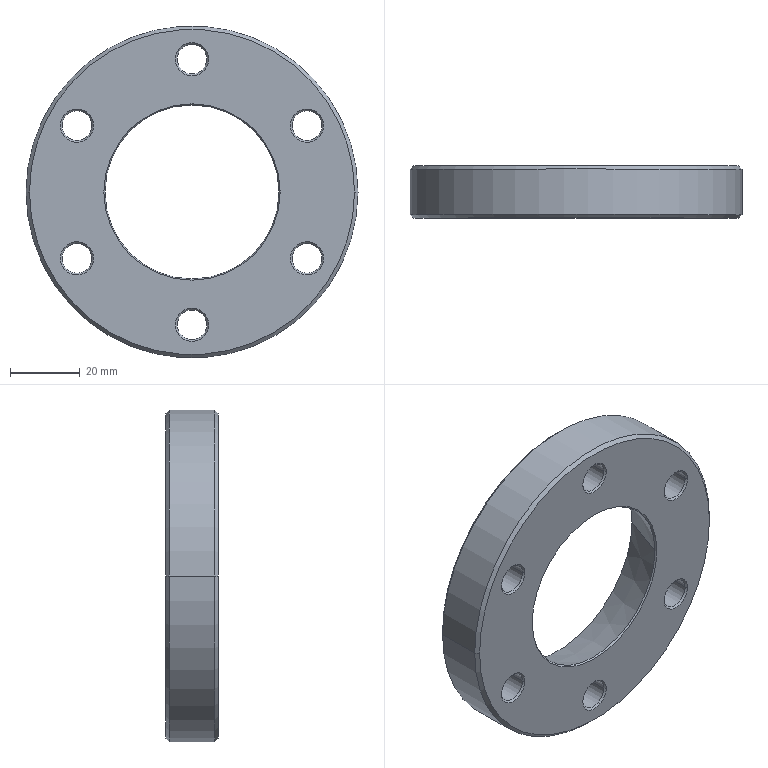Part | Creo | features CUT 7, CURVE 3, DATUM PLANE 3, CHAMFER 2, COORDINATE SYSTEM 1, PATTERN 1, PROTRUSION 1 | 1 solid | 66 faces | box 95 x 15 x 95 mm | volume 60557 mm3 | cone 32 | cylinder 26 | plane 8 | commonest cylinder face diameters 8.5 x12 14 x12 95 x2